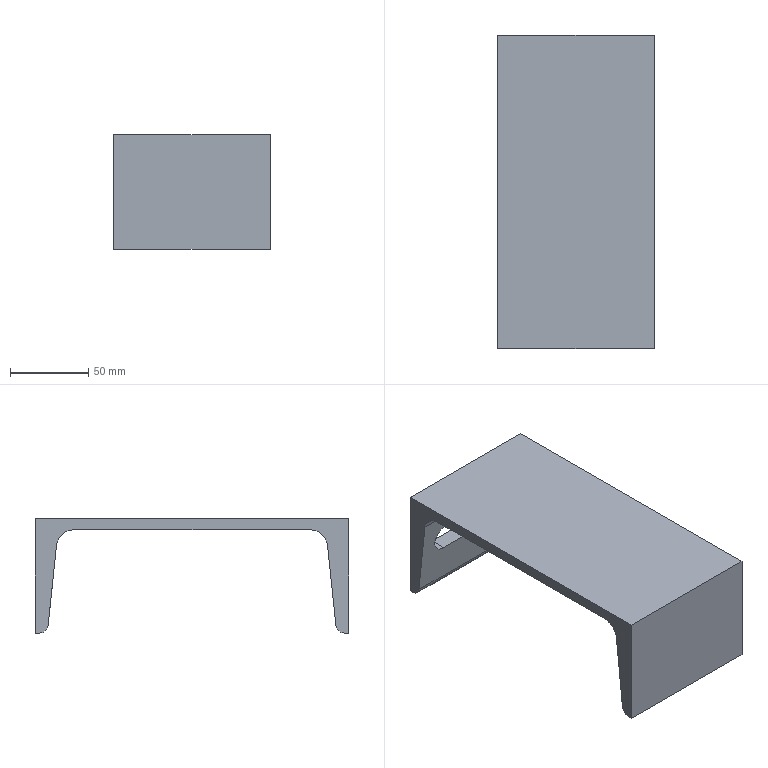Part | SolidWorks | features 3DProfileFeature 1, ICE 1, WeldMemberFeat 1, WeldmentFeature 1 | 1 solid | 18 faces | box 100 x 200 x 73 mm | volume 272858 mm3 | plane 12 | cylinder 6 | commonest cylinder face diameters 11 x2 18 x2 22 x2
STEP:
#1=CARTESIAN_POINT('',(0.,191.951,-68.075));
#2=VERTEX_POINT('',#1);
#3=CARTESIAN_POINT('',(0.,197.421,-73.));
#4=VERTEX_POINT('',#3);
#5=CARTESIAN_POINT('',(0.,197.421,-67.5));
#6=DIRECTION('',(1.,0.,0.));
#7=DIRECTION('',(0.,0.,-1.));
#8=AXIS2_PLACEMENT_3D('',#5,#6,#7);
#9=CIRCLE('',#8,5.5);
#10=EDGE_CURVE('',#2,#4,#9,.T.);
#11=ORIENTED_EDGE('',*,*,#10,.T.);
#12=CARTESIAN_POINT('',(100.,197.421,-73.));
#13=VERTEX_POINT('',#12);
#14=CARTESIAN_POINT('',(100.,197.421,-73.));
#15=DIRECTION('',(-1.,0.,0.));
#16=VECTOR('',#15,1000.);
#17=LINE('',#14,#16);
#18=EDGE_CURVE('',#13,#4,#17,.T.);
#19=ORIENTED_EDGE('',*,*,#18,.F.);
#20=CARTESIAN_POINT('',(100.,191.951,-68.075));
#21=VERTEX_POINT('',#20);
#22=CARTESIAN_POINT('',(100.,197.421,-67.5));
#23=DIRECTION('',(1.,0.,0.));
#24=DIRECTION('',(0.,0.,-1.));
#25=AXIS2_PLACEMENT_3D('',#22,#23,#24);
#26=CIRCLE('',#25,5.5);
#27=EDGE_CURVE('',#21,#13,#26,.T.);
#28=ORIENTED_EDGE('',*,*,#27,.F.);
#29=CARTESIAN_POINT('',(100.,191.951,-68.075));
#30=DIRECTION('',(-1.,0.,0.));
#31=VECTOR('',#30,1000.);
#32=LINE('',#29,#31);
#33=EDGE_CURVE('',#21,#2,#32,.T.);
#34=ORIENTED_EDGE('',*,*,#33,.T.);
#35=EDGE_LOOP('',(#11,#19,#28,#34));
#36=FACE_OUTER_BOUND('',#35,.T.);
#37=CARTESIAN_POINT('',(100.,197.421,-67.5));
#38=DIRECTION('',(-1.,0.,0.));
#39=DIRECTION('',(0.,0.,1.));
#40=AXIS2_PLACEMENT_3D('',#37,#38,#39);
#41=CYLINDRICAL_SURFACE('',#40,5.5);
#42=ADVANCED_FACE('',(#36),#41,.T.);
#43=CARTESIAN_POINT('',(0.,200.,-73.));
#44=VERTEX_POINT('',#43);
#45=CARTESIAN_POINT('',(0.,200.,-73.));
#46=DIRECTION('',(0.,1.,0.));
#47=VECTOR('',#46,1000.);
#48=LINE('',#45,#47);
#49=EDGE_CURVE('',#4,#44,#48,.T.);
#50=ORIENTED_EDGE('',*,*,#49,.T.);
#51=CARTESIAN_POINT('',(100.,200.,-73.));
#52=VERTEX_POINT('',#51);
#53=CARTESIAN_POINT('',(100.,200.,-73.));
#54=DIRECTION('',(-1.,0.,0.));
#55=VECTOR('',#54,1000.);
#56=LINE('',#53,#55);
#57=EDGE_CURVE('',#52,#44,#56,.T.);
#58=ORIENTED_EDGE('',*,*,#57,.F.);
#59=CARTESIAN_POINT('',(100.,200.,-73.));
#60=DIRECTION('',(0.,1.,0.));
#61=VECTOR('',#60,1000.);
#62=LINE('',#59,#61);
#63=EDGE_CURVE('',#13,#52,#62,.T.);
#64=ORIENTED_EDGE('',*,*,#63,.F.);
#65=ORIENTED_EDGE('',*,*,#18,.T.);
#66=EDGE_LOOP('',(#50,#58,#64,#65));
#67=FACE_OUTER_BOUND('',#66,.T.);
#68=CARTESIAN_POINT('',(100.,200.,-73.));
#69=DIRECTION('',(0.,0.,1.));
#70=DIRECTION('',(1.,0.,0.));
#71=AXIS2_PLACEMENT_3D('',#68,#69,#70);
#72=PLANE('',#71);
#73=ADVANCED_FACE('',(#67),#72,.F.);
#74=CARTESIAN_POINT('',(20.,200.,-26.));
#75=VERTEX_POINT('',#74);
#76=CARTESIAN_POINT('',(80.,200.,-26.));
#77=VERTEX_POINT('',#76);
#78=CARTESIAN_POINT('',(20.,200.,-26.));
#79=DIRECTION('',(1.,0.,0.));
#80=VECTOR('',#79,1000.);
#81=LINE('',#78,#80);
#82=EDGE_CURVE('',#75,#77,#81,.T.);
#83=ORIENTED_EDGE('',*,*,#82,.F.);
#84=CARTESIAN_POINT('',(20.,200.,-44.));
#85=VERTEX_POINT('',#84);
#86=CARTESIAN_POINT('',(20.,200.,-35.));
#87=DIRECTION('',(0.,1.,0.));
#88=DIRECTION('',(0.,0.,1.));
#89=AXIS2_PLACEMENT_3D('',#86,#87,#88);
#90=CIRCLE('',#89,9.);
#91=EDGE_CURVE('',#85,#75,#90,.T.);
#92=ORIENTED_EDGE('',*,*,#91,.F.);
#93=CARTESIAN_POINT('',(80.,200.,-44.));
#94=VERTEX_POINT('',#93);
#95=CARTESIAN_POINT('',(20.,200.,-44.));
#96=DIRECTION('',(-1.,0.,0.));
#97=VECTOR('',#96,1000.);
#98=LINE('',#95,#97);
#99=EDGE_CURVE('',#94,#85,#98,.T.);
#100=ORIENTED_EDGE('',*,*,#99,.F.);
#101=CARTESIAN_POINT('',(80.,200.,-35.));
#102=DIRECTION('',(0.,1.,0.));
#103=DIRECTION('',(0.,0.,1.));
#104=AXIS2_PLACEMENT_3D('',#101,#102,#103);
#105=CIRCLE('',#104,9.);
#106=EDGE_CURVE('',#77,#94,#105,.T.);
#107=ORIENTED_EDGE('',*,*,#106,.F.);
#108=EDGE_LOOP('',(#83,#92,#100,#107));
#109=FACE_BOUND('',#108,.T.);
#110=CARTESIAN_POINT('',(0.,200.,0.));
#111=VERTEX_POINT('',#110);
#112=CARTESIAN_POINT('',(0.,200.,-73.));
#113=DIRECTION('',(0.,0.,1.));
#114=VECTOR('',#113,1000.);
#115=LINE('',#112,#114);
#116=EDGE_CURVE('',#44,#111,#115,.T.);
#117=ORIENTED_EDGE('',*,*,#116,.T.);
#118=CARTESIAN_POINT('',(100.,200.,0.));
#119=VERTEX_POINT('',#118);
#120=CARTESIAN_POINT('',(100.,200.,0.));
#121=DIRECTION('',(-1.,0.,0.));
#122=VECTOR('',#121,1000.);
#123=LINE('',#120,#122);
#124=EDGE_CURVE('',#119,#111,#123,.T.);
#125=ORIENTED_EDGE('',*,*,#124,.F.);
#126=CARTESIAN_POINT('',(100.,200.,-73.));
#127=DIRECTION('',(0.,0.,1.));
#128=VECTOR('',#127,1000.);
#129=LINE('',#126,#128);
#130=EDGE_CURVE('',#52,#119,#129,.T.);
#131=ORIENTED_EDGE('',*,*,#130,.F.);
#132=ORIENTED_EDGE('',*,*,#57,.T.);
#133=EDGE_LOOP('',(#117,#125,#131,#132));
#134=FACE_OUTER_BOUND('',#133,.T.);
#135=CARTESIAN_POINT('',(100.,200.,-73.));
#136=DIRECTION('',(0.,-1.,0.));
#137=DIRECTION('',(0.,0.,-1.));
#138=AXIS2_PLACEMENT_3D('',#135,#136,#137);
#139=PLANE('',#138);
#140=ADVANCED_FACE('',(#109,#134),#139,.F.);
#141=CARTESIAN_POINT('',(0.,0.,0.));
#142=VERTEX_POINT('',#141);
#143=CARTESIAN_POINT('',(0.,200.,0.));
#144=DIRECTION('',(0.,-1.,0.));
#145=VECTOR('',#144,1000.);
#146=LINE('',#143,#145);
#147=EDGE_CURVE('',#111,#142,#146,.T.);
#148=ORIENTED_EDGE('',*,*,#147,.T.);
#149=CARTESIAN_POINT('',(100.,0.,0.));
#150=VERTEX_POINT('',#149);
#151=CARTESIAN_POINT('',(100.,0.,0.));
#152=DIRECTION('',(-1.,0.,0.));
#153=VECTOR('',#152,1000.);
#154=LINE('',#151,#153);
#155=EDGE_CURVE('',#150,#142,#154,.T.);
#156=ORIENTED_EDGE('',*,*,#155,.F.);
#157=CARTESIAN_POINT('',(100.,200.,0.));
#158=DIRECTION('',(0.,-1.,0.));
#159=VECTOR('',#158,1000.);
#160=LINE('',#157,#159);
#161=EDGE_CURVE('',#119,#150,#160,.T.);
#162=ORIENTED_EDGE('',*,*,#161,.F.);
#163=ORIENTED_EDGE('',*,*,#124,.T.);
#164=EDGE_LOOP('',(#148,#156,#162,#163));
#165=FACE_OUTER_BOUND('',#164,.T.);
#166=CARTESIAN_POINT('',(100.,200.,0.));
#167=DIRECTION('',(0.,0.,-1.));
#168=DIRECTION('',(-1.,0.,0.));
#169=AXIS2_PLACEMENT_3D('',#166,#167,#168);
#170=PLANE('',#169);
#171=ADVANCED_FACE('',(#165),#170,.F.);
#172=CARTESIAN_POINT('',(0.,0.,-73.));
#173=VERTEX_POINT('',#172);
#174=CARTESIAN_POINT('',(0.,0.,-73.));
#175=DIRECTION('',(0.,0.,-1.));
#176=VECTOR('',#175,1000.);
#177=LINE('',#174,#176);
#178=EDGE_CURVE('',#142,#173,#177,.T.);
#179=ORIENTED_EDGE('',*,*,#178,.T.);
#180=CARTESIAN_POINT('',(100.,0.,-73.));
#181=VERTEX_POINT('',#180);
#182=CARTESIAN_POINT('',(100.,0.,-73.));
#183=DIRECTION('',(-1.,0.,0.));
#184=VECTOR('',#183,1000.);
#185=LINE('',#182,#184);
#186=EDGE_CURVE('',#181,#173,#185,.T.);
#187=ORIENTED_EDGE('',*,*,#186,.F.);
#188=CARTESIAN_POINT('',(100.,0.,-73.));
#189=DIRECTION('',(0.,0.,-1.));
#190=VECTOR('',#189,1000.);
#191=LINE('',#188,#190);
#192=EDGE_CURVE('',#150,#181,#191,.T.);
#193=ORIENTED_EDGE('',*,*,#192,.F.);
#194=ORIENTED_EDGE('',*,*,#155,.T.);
#195=EDGE_LOOP('',(#179,#187,#193,#194));
#196=FACE_OUTER_BOUND('',#195,.T.);
#197=CARTESIAN_POINT('',(100.,0.,-73.));
#198=DIRECTION('',(0.,1.,0.));
#199=DIRECTION('',(0.,0.,1.));
#200=AXIS2_PLACEMENT_3D('',#197,#198,#199);
#201=PLANE('',#200);
#202=ADVANCED_FACE('',(#196),#201,.F.);
#203=CARTESIAN_POINT('',(0.,2.579,-73.));
#204=VERTEX_POINT('',#203);
#205=CARTESIAN_POINT('',(0.,0.,-73.));
#206=DIRECTION('',(0.,1.,0.));
#207=VECTOR('',#206,1000.);
#208=LINE('',#205,#207);
#209=EDGE_CURVE('',#173,#204,#208,.T.);
#210=ORIENTED_EDGE('',*,*,#209,.T.);
#211=CARTESIAN_POINT('',(100.,2.579,-73.));
#212=VERTEX_POINT('',#211);
#213=CARTESIAN_POINT('',(100.,2.579,-73.));
#214=DIRECTION('',(-1.,0.,0.));
#215=VECTOR('',#214,1000.);
#216=LINE('',#213,#215);
#217=EDGE_CURVE('',#212,#204,#216,.T.);
#218=ORIENTED_EDGE('',*,*,#217,.F.);
#219=CARTESIAN_POINT('',(100.,0.,-73.));
#220=DIRECTION('',(0.,1.,0.));
#221=VECTOR('',#220,1000.);
#222=LINE('',#219,#221);
#223=EDGE_CURVE('',#181,#212,#222,.T.);
#224=ORIENTED_EDGE('',*,*,#223,.F.);
#225=ORIENTED_EDGE('',*,*,#186,.T.);
#226=EDGE_LOOP('',(#210,#218,#224,#225));
#227=FACE_OUTER_BOUND('',#226,.T.);
#228=CARTESIAN_POINT('',(100.,0.,-73.));
#229=DIRECTION('',(0.,0.,1.));
#230=DIRECTION('',(1.,0.,0.));
#231=AXIS2_PLACEMENT_3D('',#228,#229,#230);
#232=PLANE('',#231);
#233=ADVANCED_FACE('',(#227),#232,.F.);
#234=CARTESIAN_POINT('',(0.,8.049,-68.075));
#235=VERTEX_POINT('',#234);
#236=CARTESIAN_POINT('',(0.,2.579,-67.5));
#237=DIRECTION('',(1.,0.,0.));
#238=DIRECTION('',(0.,0.,1.));
#239=AXIS2_PLACEMENT_3D('',#236,#237,#238);
#240=CIRCLE('',#239,5.5);
#241=EDGE_CURVE('',#204,#235,#240,.T.);
#242=ORIENTED_EDGE('',*,*,#241,.T.);
#243=CARTESIAN_POINT('',(100.,8.049,-68.075));
#244=VERTEX_POINT('',#243);
#245=CARTESIAN_POINT('',(100.,8.049,-68.075));
#246=DIRECTION('',(-1.,0.,0.));
#247=VECTOR('',#246,1000.);
#248=LINE('',#245,#247);
#249=EDGE_CURVE('',#244,#235,#248,.T.);
#250=ORIENTED_EDGE('',*,*,#249,.F.);
#251=CARTESIAN_POINT('',(100.,2.579,-67.5));
#252=DIRECTION('',(1.,0.,0.));
#253=DIRECTION('',(0.,0.,1.));
#254=AXIS2_PLACEMENT_3D('',#251,#252,#253);
#255=CIRCLE('',#254,5.5);
#256=EDGE_CURVE('',#212,#244,#255,.T.);
#257=ORIENTED_EDGE('',*,*,#256,.F.);
#258=ORIENTED_EDGE('',*,*,#217,.T.);
#259=EDGE_LOOP('',(#242,#250,#257,#258));
#260=FACE_OUTER_BOUND('',#259,.T.);
#261=CARTESIAN_POINT('',(100.,2.579,-67.5));
#262=DIRECTION('',(-1.,0.,0.));
#263=DIRECTION('',(0.,0.,1.));
#264=AXIS2_PLACEMENT_3D('',#261,#262,#263);
#265=CYLINDRICAL_SURFACE('',#264,5.5);
#266=ADVANCED_FACE('',(#260),#265,.T.);
#267=CARTESIAN_POINT('',(0.,13.433,-16.85));
#268=VERTEX_POINT('',#267);
#269=CARTESIAN_POINT('',(0.,13.433,-16.85));
#270=DIRECTION('',(0.,0.1045,0.9945));
#271=VECTOR('',#270,1000.);
#272=LINE('',#269,#271);
#273=EDGE_CURVE('',#235,#268,#272,.T.);
#274=ORIENTED_EDGE('',*,*,#273,.T.);
#275=CARTESIAN_POINT('',(100.,13.433,-16.85));
#276=VERTEX_POINT('',#275);
#277=CARTESIAN_POINT('',(100.,13.433,-16.85));
#278=DIRECTION('',(-1.,0.,0.));
#279=VECTOR('',#278,1000.);
#280=LINE('',#277,#279);
#281=EDGE_CURVE('',#276,#268,#280,.T.);
#282=ORIENTED_EDGE('',*,*,#281,.F.);
#283=CARTESIAN_POINT('',(100.,13.433,-16.85));
#284=DIRECTION('',(0.,0.1045,0.9945));
#285=VECTOR('',#284,1000.);
#286=LINE('',#283,#285);
#287=EDGE_CURVE('',#244,#276,#286,.T.);
#288=ORIENTED_EDGE('',*,*,#287,.F.);
#289=ORIENTED_EDGE('',*,*,#249,.T.);
#290=EDGE_LOOP('',(#274,#282,#288,#289));
#291=FACE_OUTER_BOUND('',#290,.T.);
#292=CARTESIAN_POINT('',(100.,13.433,-16.85));
#293=DIRECTION('',(0.,-0.9945,0.1045));
#294=DIRECTION('',(0.,-0.1045,-0.9945));
#295=AXIS2_PLACEMENT_3D('',#292,#293,#294);
#296=PLANE('',#295);
#297=ADVANCED_FACE('',(#291),#296,.F.);
#298=CARTESIAN_POINT('',(0.,24.373,-7.));
#299=VERTEX_POINT('',#298);
#300=CARTESIAN_POINT('',(0.,24.373,-18.));
#301=DIRECTION('',(-1.,0.,0.));
#302=DIRECTION('',(0.,0.,-1.));
#303=AXIS2_PLACEMENT_3D('',#300,#301,#302);
#304=CIRCLE('',#303,11.);
#305=EDGE_CURVE('',#268,#299,#304,.T.);
#306=ORIENTED_EDGE('',*,*,#305,.T.);
#307=CARTESIAN_POINT('',(100.,24.373,-7.));
#308=VERTEX_POINT('',#307);
#309=CARTESIAN_POINT('',(100.,24.373,-7.));
#310=DIRECTION('',(-1.,0.,0.));
#311=VECTOR('',#310,1000.);
#312=LINE('',#309,#311);
#313=EDGE_CURVE('',#308,#299,#312,.T.);
#314=ORIENTED_EDGE('',*,*,#313,.F.);
#315=CARTESIAN_POINT('',(100.,24.373,-18.));
#316=DIRECTION('',(-1.,0.,0.));
#317=DIRECTION('',(0.,0.,-1.));
#318=AXIS2_PLACEMENT_3D('',#315,#316,#317);
#319=CIRCLE('',#318,11.);
#320=EDGE_CURVE('',#276,#308,#319,.T.);
#321=ORIENTED_EDGE('',*,*,#320,.F.);
#322=ORIENTED_EDGE('',*,*,#281,.T.);
#323=EDGE_LOOP('',(#306,#314,#321,#322));
#324=FACE_OUTER_BOUND('',#323,.T.);
#325=CARTESIAN_POINT('',(100.,24.373,-18.));
#326=DIRECTION('',(-1.,0.,0.));
#327=DIRECTION('',(0.,0.,1.));
#328=AXIS2_PLACEMENT_3D('',#325,#326,#327);
#329=CYLINDRICAL_SURFACE('',#328,11.);
#330=ADVANCED_FACE('',(#324),#329,.F.);
#331=CARTESIAN_POINT('',(0.,175.627,-7.));
#332=VERTEX_POINT('',#331);
#333=CARTESIAN_POINT('',(0.,175.627,-7.));
#334=DIRECTION('',(0.,1.,0.));
#335=VECTOR('',#334,1000.);
#336=LINE('',#333,#335);
#337=EDGE_CURVE('',#299,#332,#336,.T.);
#338=ORIENTED_EDGE('',*,*,#337,.T.);
#339=CARTESIAN_POINT('',(100.,175.627,-7.));
#340=VERTEX_POINT('',#339);
#341=CARTESIAN_POINT('',(100.,175.627,-7.));
#342=DIRECTION('',(-1.,0.,0.));
#343=VECTOR('',#342,1000.);
#344=LINE('',#341,#343);
#345=EDGE_CURVE('',#340,#332,#344,.T.);
#346=ORIENTED_EDGE('',*,*,#345,.F.);
#347=CARTESIAN_POINT('',(100.,175.627,-7.));
#348=DIRECTION('',(0.,1.,0.));
#349=VECTOR('',#348,1000.);
#350=LINE('',#347,#349);
#351=EDGE_CURVE('',#308,#340,#350,.T.);
#352=ORIENTED_EDGE('',*,*,#351,.F.);
#353=ORIENTED_EDGE('',*,*,#313,.T.);
#354=EDGE_LOOP('',(#338,#346,#352,#353));
#355=FACE_OUTER_BOUND('',#354,.T.);
#356=CARTESIAN_POINT('',(100.,175.627,-7.));
#357=DIRECTION('',(0.,0.,1.));
#358=DIRECTION('',(1.,0.,0.));
#359=AXIS2_PLACEMENT_3D('',#356,#357,#358);
#360=PLANE('',#359);
#361=ADVANCED_FACE('',(#355),#360,.F.);
#362=CARTESIAN_POINT('',(0.,186.567,-16.85));
#363=VERTEX_POINT('',#362);
#364=CARTESIAN_POINT('',(0.,175.627,-18.));
#365=DIRECTION('',(-1.,0.,0.));
#366=DIRECTION('',(0.,0.,1.));
#367=AXIS2_PLACEMENT_3D('',#364,#365,#366);
#368=CIRCLE('',#367,11.);
#369=EDGE_CURVE('',#332,#363,#368,.T.);
#370=ORIENTED_EDGE('',*,*,#369,.T.);
#371=CARTESIAN_POINT('',(100.,186.567,-16.85));
#372=VERTEX_POINT('',#371);
#373=CARTESIAN_POINT('',(100.,186.567,-16.85));
#374=DIRECTION('',(-1.,0.,0.));
#375=VECTOR('',#374,1000.);
#376=LINE('',#373,#375);
#377=EDGE_CURVE('',#372,#363,#376,.T.);
#378=ORIENTED_EDGE('',*,*,#377,.F.);
#379=CARTESIAN_POINT('',(100.,175.627,-18.));
#380=DIRECTION('',(-1.,0.,0.));
#381=DIRECTION('',(0.,0.,1.));
#382=AXIS2_PLACEMENT_3D('',#379,#380,#381);
#383=CIRCLE('',#382,11.);
#384=EDGE_CURVE('',#340,#372,#383,.T.);
#385=ORIENTED_EDGE('',*,*,#384,.F.);
#386=ORIENTED_EDGE('',*,*,#345,.T.);
#387=EDGE_LOOP('',(#370,#378,#385,#386));
#388=FACE_OUTER_BOUND('',#387,.T.);
#389=CARTESIAN_POINT('',(100.,175.627,-18.));
#390=DIRECTION('',(-1.,0.,0.));
#391=DIRECTION('',(0.,0.,1.));
#392=AXIS2_PLACEMENT_3D('',#389,#390,#391);
#393=CYLINDRICAL_SURFACE('',#392,11.);
#394=ADVANCED_FACE('',(#388),#393,.F.);
#395=CARTESIAN_POINT('',(80.,189.42,-44.));
#396=VERTEX_POINT('',#395);
#397=CARTESIAN_POINT('',(20.,189.42,-44.));
#398=VERTEX_POINT('',#397);
#399=CARTESIAN_POINT('',(100.,189.42,-44.));
#400=DIRECTION('',(-1.,0.,0.));
#401=VECTOR('',#400,1000.);
#402=LINE('',#399,#401);
#403=EDGE_CURVE('',#396,#398,#402,.T.);
#404=ORIENTED_EDGE('',*,*,#403,.T.);
#405=CARTESIAN_POINT('',(20.,187.529,-26.));
#406=VERTEX_POINT('',#405);
#407=CARTESIAN_POINT('',(20.,189.42,-44.));
#408=CARTESIAN_POINT('',(2.,189.42,-44.));
#409=CARTESIAN_POINT('',(2.,187.529,-26.));
#410=CARTESIAN_POINT('',(20.,187.529,-26.));
#411=(BOUNDED_CURVE()B_SPLINE_CURVE(3,(#407,#408,#409,#410),.UNSPECIFIED.,.F.,.F.)B_SPLINE_CURVE_WITH_KNOTS((4,4),(0.,3.142),.UNSPECIFIED.)CURVE()GEOMETRIC_REPRESENTATION_ITEM()RATIONAL_B_SPLINE_CURVE((1.,0.3333,0.3333,1.))REPRESENTATION_ITEM(''));
#412=EDGE_CURVE('',#398,#406,#411,.T.);
#413=ORIENTED_EDGE('',*,*,#412,.T.);
#414=CARTESIAN_POINT('',(80.,187.529,-26.));
#415=VERTEX_POINT('',#414);
#416=CARTESIAN_POINT('',(100.,187.529,-26.));
#417=DIRECTION('',(1.,0.,0.));
#418=VECTOR('',#417,1000.);
#419=LINE('',#416,#418);
#420=EDGE_CURVE('',#406,#415,#419,.T.);
#421=ORIENTED_EDGE('',*,*,#420,.T.);
#422=CARTESIAN_POINT('',(80.,187.529,-26.));
#423=CARTESIAN_POINT('',(98.,187.529,-26.));
#424=CARTESIAN_POINT('',(98.,189.42,-44.));
#425=CARTESIAN_POINT('',(80.,189.42,-44.));
#426=(BOUNDED_CURVE()B_SPLINE_CURVE(3,(#422,#423,#424,#425),.UNSPECIFIED.,.F.,.F.)B_SPLINE_CURVE_WITH_KNOTS((4,4),(3.142,6.283),.UNSPECIFIED.)CURVE()GEOMETRIC_REPRESENTATION_ITEM()RATIONAL_B_SPLINE_CURVE((1.,0.3333,0.3333,1.))REPRESENTATION_ITEM(''));
#427=EDGE_CURVE('',#415,#396,#426,.T.);
#428=ORIENTED_EDGE('',*,*,#427,.T.);
#429=EDGE_LOOP('',(#404,#413,#421,#428));
#430=FACE_BOUND('',#429,.T.);
#431=CARTESIAN_POINT('',(0.,186.567,-16.85));
#432=DIRECTION('',(0.,0.1045,-0.9945));
#433=VECTOR('',#432,1000.);
#434=LINE('',#431,#433);
#435=EDGE_CURVE('',#363,#2,#434,.T.);
#436=ORIENTED_EDGE('',*,*,#435,.T.);
#437=ORIENTED_EDGE('',*,*,#33,.F.);
#438=CARTESIAN_POINT('',(100.,186.567,-16.85));
#439=DIRECTION('',(0.,0.1045,-0.9945));
#440=VECTOR('',#439,1000.);
#441=LINE('',#438,#440);
#442=EDGE_CURVE('',#372,#21,#441,.T.);
#443=ORIENTED_EDGE('',*,*,#442,.F.);
#444=ORIENTED_EDGE('',*,*,#377,.T.);
#445=EDGE_LOOP('',(#436,#437,#443,#444));
#446=FACE_OUTER_BOUND('',#445,.T.);
#447=CARTESIAN_POINT('',(100.,186.567,-16.85));
#448=DIRECTION('',(0.,0.9945,0.1045));
#449=DIRECTION('',(0.,-0.1045,0.9945));
#450=AXIS2_PLACEMENT_3D('',#447,#448,#449);
#451=PLANE('',#450);
#452=ADVANCED_FACE('',(#430,#446),#451,.F.);
#453=ORIENTED_EDGE('',*,*,#27,.T.);
#454=ORIENTED_EDGE('',*,*,#63,.T.);
#455=ORIENTED_EDGE('',*,*,#130,.T.);
#456=ORIENTED_EDGE('',*,*,#161,.T.);
#457=ORIENTED_EDGE('',*,*,#192,.T.);
#458=ORIENTED_EDGE('',*,*,#223,.T.);
#459=ORIENTED_EDGE('',*,*,#256,.T.);
#460=ORIENTED_EDGE('',*,*,#287,.T.);
#461=ORIENTED_EDGE('',*,*,#320,.T.);
#462=ORIENTED_EDGE('',*,*,#351,.T.);
#463=ORIENTED_EDGE('',*,*,#384,.T.);
#464=ORIENTED_EDGE('',*,*,#442,.T.);
#465=EDGE_LOOP('',(#453,#454,#455,#456,#457,#458,#459,#460,#461,#462,#463,#464));
#466=FACE_OUTER_BOUND('',#465,.T.);
#467=CARTESIAN_POINT('',(100.,197.421,-67.5));
#468=DIRECTION('',(1.,0.,0.));
#469=DIRECTION('',(0.,0.,-1.));
#470=AXIS2_PLACEMENT_3D('',#467,#468,#469);
#471=PLANE('',#470);
#472=ADVANCED_FACE('',(#466),#471,.T.);
#473=ORIENTED_EDGE('',*,*,#10,.F.);
#474=ORIENTED_EDGE('',*,*,#435,.F.);
#475=ORIENTED_EDGE('',*,*,#369,.F.);
#476=ORIENTED_EDGE('',*,*,#337,.F.);
#477=ORIENTED_EDGE('',*,*,#305,.F.);
#478=ORIENTED_EDGE('',*,*,#273,.F.);
#479=ORIENTED_EDGE('',*,*,#241,.F.);
#480=ORIENTED_EDGE('',*,*,#209,.F.);
#481=ORIENTED_EDGE('',*,*,#178,.F.);
#482=ORIENTED_EDGE('',*,*,#147,.F.);
#483=ORIENTED_EDGE('',*,*,#116,.F.);
#484=ORIENTED_EDGE('',*,*,#49,.F.);
#485=EDGE_LOOP('',(#473,#474,#475,#476,#477,#478,#479,#480,#481,#482,#483,#484));
#486=FACE_OUTER_BOUND('',#485,.T.);
#487=CARTESIAN_POINT('',(0.,197.421,-67.5));
#488=DIRECTION('',(1.,0.,0.));
#489=DIRECTION('',(0.,0.,-1.));
#490=AXIS2_PLACEMENT_3D('',#487,#488,#489);
#491=PLANE('',#490);
#492=ADVANCED_FACE('',(#486),#491,.F.);
#493=CARTESIAN_POINT('',(20.,184.,-44.));
#494=DIRECTION('',(0.,1.,0.));
#495=VECTOR('',#494,1000.);
#496=LINE('',#493,#495);
#497=EDGE_CURVE('',#398,#85,#496,.T.);
#498=ORIENTED_EDGE('',*,*,#497,.T.);
#499=ORIENTED_EDGE('',*,*,#91,.T.);
#500=CARTESIAN_POINT('',(20.,184.,-26.));
#501=DIRECTION('',(0.,1.,0.));
#502=VECTOR('',#501,1000.);
#503=LINE('',#500,#502);
#504=EDGE_CURVE('',#406,#75,#503,.T.);
#505=ORIENTED_EDGE('',*,*,#504,.F.);
#506=ORIENTED_EDGE('',*,*,#412,.F.);
#507=EDGE_LOOP('',(#498,#499,#505,#506));
#508=FACE_OUTER_BOUND('',#507,.T.);
#509=CARTESIAN_POINT('',(20.,184.,-35.));
#510=DIRECTION('',(0.,1.,0.));
#511=DIRECTION('',(0.,0.,1.));
#512=AXIS2_PLACEMENT_3D('',#509,#510,#511);
#513=CYLINDRICAL_SURFACE('',#512,9.);
#514=ADVANCED_FACE('',(#508),#513,.F.);
#515=CARTESIAN_POINT('',(80.,184.,-44.));
#516=DIRECTION('',(0.,1.,0.));
#517=VECTOR('',#516,1000.);
#518=LINE('',#515,#517);
#519=EDGE_CURVE('',#396,#94,#518,.T.);
#520=ORIENTED_EDGE('',*,*,#519,.T.);
#521=ORIENTED_EDGE('',*,*,#99,.T.);
#522=ORIENTED_EDGE('',*,*,#497,.F.);
#523=ORIENTED_EDGE('',*,*,#403,.F.);
#524=EDGE_LOOP('',(#520,#521,#522,#523));
#525=FACE_OUTER_BOUND('',#524,.T.);
#526=CARTESIAN_POINT('',(20.,184.,-44.));
#527=DIRECTION('',(0.,0.,-1.));
#528=DIRECTION('',(-1.,0.,0.));
#529=AXIS2_PLACEMENT_3D('',#526,#527,#528);
#530=PLANE('',#529);
#531=ADVANCED_FACE('',(#525),#530,.F.);
#532=CARTESIAN_POINT('',(80.,184.,-26.));
#533=DIRECTION('',(0.,1.,0.));
#534=VECTOR('',#533,1000.);
#535=LINE('',#532,#534);
#536=EDGE_CURVE('',#415,#77,#535,.T.);
#537=ORIENTED_EDGE('',*,*,#536,.T.);
#538=ORIENTED_EDGE('',*,*,#106,.T.);
#539=ORIENTED_EDGE('',*,*,#519,.F.);
#540=ORIENTED_EDGE('',*,*,#427,.F.);
#541=EDGE_LOOP('',(#537,#538,#539,#540));
#542=FACE_OUTER_BOUND('',#541,.T.);
#543=CARTESIAN_POINT('',(80.,184.,-35.));
#544=DIRECTION('',(0.,1.,0.));
#545=DIRECTION('',(0.,0.,1.));
#546=AXIS2_PLACEMENT_3D('',#543,#544,#545);
#547=CYLINDRICAL_SURFACE('',#546,9.);
#548=ADVANCED_FACE('',(#542),#547,.F.);
#549=ORIENTED_EDGE('',*,*,#504,.T.);
#550=ORIENTED_EDGE('',*,*,#82,.T.);
#551=ORIENTED_EDGE('',*,*,#536,.F.);
#552=ORIENTED_EDGE('',*,*,#420,.F.);
#553=EDGE_LOOP('',(#549,#550,#551,#552));
#554=FACE_OUTER_BOUND('',#553,.T.);
#555=CARTESIAN_POINT('',(20.,184.,-26.));
#556=DIRECTION('',(0.,0.,1.));
#557=DIRECTION('',(1.,0.,0.));
#558=AXIS2_PLACEMENT_3D('',#555,#556,#557);
#559=PLANE('',#558);
#560=ADVANCED_FACE('',(#554),#559,.F.);
#561=CLOSED_SHELL('',(#42,#73,#140,#171,#202,#233,#266,#297,#330,#361,#394,#452,#472,#492,#514,#531,#548,#560));
#562=MANIFOLD_SOLID_BREP('',#561);
#563=CARTESIAN_POINT('',(0.,0.,0.));
#564=DIRECTION('',(0.,0.,1.));
#565=DIRECTION('',(1.,0.,0.));
#566=AXIS2_PLACEMENT_3D('',#563,#564,#565);
#567=(LENGTH_UNIT()NAMED_UNIT(*)SI_UNIT(.MILLI.,.METRE.));
#568=UNCERTAINTY_MEASURE_WITH_UNIT(LENGTH_MEASURE(0.00001),#567,'','');
#569=(NAMED_UNIT(*)PLANE_ANGLE_UNIT()SI_UNIT($,.RADIAN.));
#570=(NAMED_UNIT(*)SI_UNIT($,.STERADIAN.)SOLID_ANGLE_UNIT());
#571=(GEOMETRIC_REPRESENTATION_CONTEXT(3)GLOBAL_UNCERTAINTY_ASSIGNED_CONTEXT((#568))GLOBAL_UNIT_ASSIGNED_CONTEXT((#567,#569,#570))REPRESENTATION_CONTEXT('',''));
#572=ADVANCED_BREP_SHAPE_REPRESENTATION('',(#562,#566),#571);